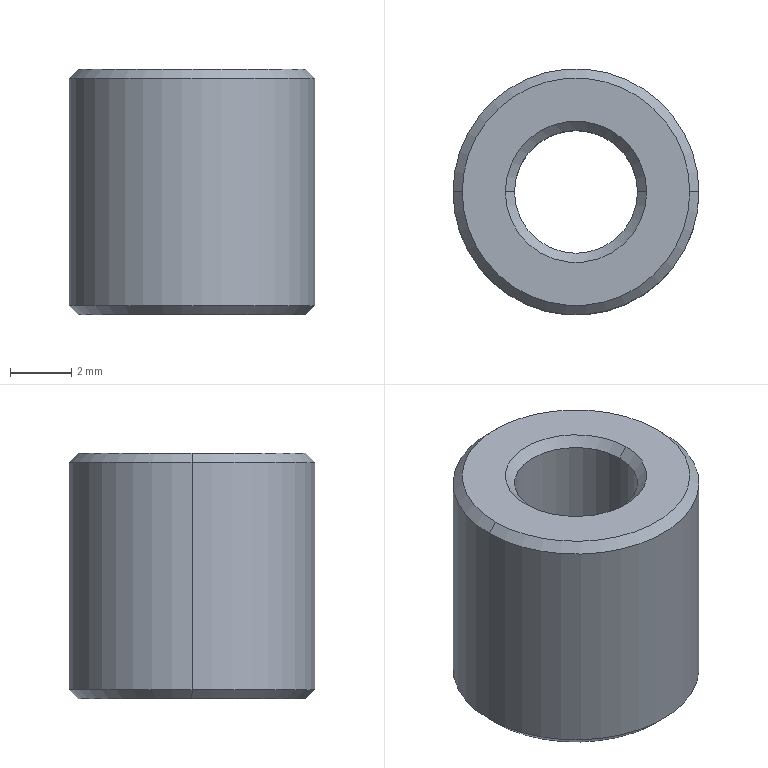Part | SolidWorks | features Chamfer 1, Extrusion 1 | 1 solid | 14 faces | box 8 x 8 x 8 mm | volume 298.2 mm3 | cone 8 | cylinder 4 | plane 2 | commonest cylinder face diameters 4 x2 8 x2
STEP:
#1=CARTESIAN_POINT('',(3.7,0.,8.));
#2=VERTEX_POINT('',#1);
#3=CARTESIAN_POINT('',(-3.7,0.,8.));
#4=VERTEX_POINT('',#3);
#5=CARTESIAN_POINT('',(0.,0.,8.));
#6=DIRECTION('',(0.,0.,1.));
#7=DIRECTION('',(1.,0.,0.));
#8=AXIS2_PLACEMENT_3D('',#5,#6,#7);
#9=CIRCLE('',#8,3.7);
#10=EDGE_CURVE('',#2,#4,#9,.T.);
#11=ORIENTED_EDGE('',*,*,#10,.F.);
#12=CARTESIAN_POINT('',(4.,0.,7.7));
#13=VERTEX_POINT('',#12);
#14=CARTESIAN_POINT('',(3.7,0.,8.));
#15=DIRECTION('',(0.7071,0.,-0.7071));
#16=VECTOR('',#15,1000.);
#17=LINE('',#14,#16);
#18=EDGE_CURVE('',#2,#13,#17,.T.);
#19=ORIENTED_EDGE('',*,*,#18,.T.);
#20=CARTESIAN_POINT('',(-4.,0.,7.7));
#21=VERTEX_POINT('',#20);
#22=CARTESIAN_POINT('',(0.,0.,7.7));
#23=DIRECTION('',(0.,0.,-1.));
#24=DIRECTION('',(1.,0.,0.));
#25=AXIS2_PLACEMENT_3D('',#22,#23,#24);
#26=CIRCLE('',#25,4.);
#27=EDGE_CURVE('',#21,#13,#26,.T.);
#28=ORIENTED_EDGE('',*,*,#27,.F.);
#29=CARTESIAN_POINT('',(-3.7,0.,8.));
#30=DIRECTION('',(-0.7071,0.,-0.7071));
#31=VECTOR('',#30,1000.);
#32=LINE('',#29,#31);
#33=EDGE_CURVE('',#4,#21,#32,.T.);
#34=ORIENTED_EDGE('',*,*,#33,.F.);
#35=EDGE_LOOP('',(#11,#19,#28,#34));
#36=FACE_OUTER_BOUND('',#35,.T.);
#37=CARTESIAN_POINT('',(0.,0.,8.));
#38=DIRECTION('',(0.,0.,-1.));
#39=DIRECTION('',(-1.,0.,0.));
#40=AXIS2_PLACEMENT_3D('',#37,#38,#39);
#41=CONICAL_SURFACE('',#40,3.7,0.7854);
#42=ADVANCED_FACE('',(#36),#41,.T.);
#43=CARTESIAN_POINT('',(-3.7,0.,0.));
#44=VERTEX_POINT('',#43);
#45=CARTESIAN_POINT('',(3.7,0.,0.));
#46=VERTEX_POINT('',#45);
#47=CARTESIAN_POINT('',(0.,0.,0.));
#48=DIRECTION('',(0.,0.,-1.));
#49=DIRECTION('',(1.,0.,0.));
#50=AXIS2_PLACEMENT_3D('',#47,#48,#49);
#51=CIRCLE('',#50,3.7);
#52=EDGE_CURVE('',#44,#46,#51,.T.);
#53=ORIENTED_EDGE('',*,*,#52,.F.);
#54=CARTESIAN_POINT('',(-4.,0.,0.3));
#55=VERTEX_POINT('',#54);
#56=CARTESIAN_POINT('',(-4.,0.,0.3));
#57=DIRECTION('',(-0.7071,0.,0.7071));
#58=VECTOR('',#57,1000.);
#59=LINE('',#56,#58);
#60=EDGE_CURVE('',#44,#55,#59,.T.);
#61=ORIENTED_EDGE('',*,*,#60,.T.);
#62=CARTESIAN_POINT('',(4.,0.,0.3));
#63=VERTEX_POINT('',#62);
#64=CARTESIAN_POINT('',(0.,0.,0.3));
#65=DIRECTION('',(0.,0.,1.));
#66=DIRECTION('',(1.,0.,0.));
#67=AXIS2_PLACEMENT_3D('',#64,#65,#66);
#68=CIRCLE('',#67,4.);
#69=EDGE_CURVE('',#63,#55,#68,.T.);
#70=ORIENTED_EDGE('',*,*,#69,.F.);
#71=CARTESIAN_POINT('',(4.,0.,0.3));
#72=DIRECTION('',(0.7071,0.,0.7071));
#73=VECTOR('',#72,1000.);
#74=LINE('',#71,#73);
#75=EDGE_CURVE('',#46,#63,#74,.T.);
#76=ORIENTED_EDGE('',*,*,#75,.F.);
#77=EDGE_LOOP('',(#53,#61,#70,#76));
#78=FACE_OUTER_BOUND('',#77,.T.);
#79=CARTESIAN_POINT('',(0.,0.,0.3));
#80=DIRECTION('',(0.,0.,1.));
#81=DIRECTION('',(1.,0.,0.));
#82=AXIS2_PLACEMENT_3D('',#79,#80,#81);
#83=CONICAL_SURFACE('',#82,4.,0.7854);
#84=ADVANCED_FACE('',(#78),#83,.T.);
#85=CARTESIAN_POINT('',(-2.,0.,7.7));
#86=VERTEX_POINT('',#85);
#87=CARTESIAN_POINT('',(2.,0.,7.7));
#88=VERTEX_POINT('',#87);
#89=CARTESIAN_POINT('',(0.,0.,7.7));
#90=DIRECTION('',(0.,0.,1.));
#91=DIRECTION('',(1.,0.,0.));
#92=AXIS2_PLACEMENT_3D('',#89,#90,#91);
#93=CIRCLE('',#92,2.);
#94=EDGE_CURVE('',#86,#88,#93,.T.);
#95=ORIENTED_EDGE('',*,*,#94,.F.);
#96=CARTESIAN_POINT('',(-2.3,0.,8.));
#97=VERTEX_POINT('',#96);
#98=CARTESIAN_POINT('',(-2.,0.,7.7));
#99=DIRECTION('',(-0.7071,0.,0.7071));
#100=VECTOR('',#99,1000.);
#101=LINE('',#98,#100);
#102=EDGE_CURVE('',#86,#97,#101,.T.);
#103=ORIENTED_EDGE('',*,*,#102,.T.);
#104=CARTESIAN_POINT('',(2.3,0.,8.));
#105=VERTEX_POINT('',#104);
#106=CARTESIAN_POINT('',(0.,0.,8.));
#107=DIRECTION('',(0.,0.,-1.));
#108=DIRECTION('',(1.,0.,0.));
#109=AXIS2_PLACEMENT_3D('',#106,#107,#108);
#110=CIRCLE('',#109,2.3);
#111=EDGE_CURVE('',#105,#97,#110,.T.);
#112=ORIENTED_EDGE('',*,*,#111,.F.);
#113=CARTESIAN_POINT('',(2.,0.,7.7));
#114=DIRECTION('',(0.7071,0.,0.7071));
#115=VECTOR('',#114,1000.);
#116=LINE('',#113,#115);
#117=EDGE_CURVE('',#88,#105,#116,.T.);
#118=ORIENTED_EDGE('',*,*,#117,.F.);
#119=EDGE_LOOP('',(#95,#103,#112,#118));
#120=FACE_OUTER_BOUND('',#119,.T.);
#121=CARTESIAN_POINT('',(0.,0.,7.7));
#122=DIRECTION('',(0.,0.,1.));
#123=DIRECTION('',(1.,0.,0.));
#124=AXIS2_PLACEMENT_3D('',#121,#122,#123);
#125=CONICAL_SURFACE('',#124,2.,0.7854);
#126=ADVANCED_FACE('',(#120),#125,.F.);
#127=CARTESIAN_POINT('',(2.,0.,0.3));
#128=VERTEX_POINT('',#127);
#129=CARTESIAN_POINT('',(-2.,0.,0.3));
#130=VERTEX_POINT('',#129);
#131=CARTESIAN_POINT('',(0.,0.,0.3));
#132=DIRECTION('',(0.,0.,-1.));
#133=DIRECTION('',(1.,0.,0.));
#134=AXIS2_PLACEMENT_3D('',#131,#132,#133);
#135=CIRCLE('',#134,2.);
#136=EDGE_CURVE('',#128,#130,#135,.T.);
#137=ORIENTED_EDGE('',*,*,#136,.F.);
#138=CARTESIAN_POINT('',(2.3,0.,0.));
#139=VERTEX_POINT('',#138);
#140=CARTESIAN_POINT('',(2.3,0.,0.));
#141=DIRECTION('',(0.7071,0.,-0.7071));
#142=VECTOR('',#141,1000.);
#143=LINE('',#140,#142);
#144=EDGE_CURVE('',#128,#139,#143,.T.);
#145=ORIENTED_EDGE('',*,*,#144,.T.);
#146=CARTESIAN_POINT('',(-2.3,0.,0.));
#147=VERTEX_POINT('',#146);
#148=CARTESIAN_POINT('',(0.,0.,0.));
#149=DIRECTION('',(0.,0.,1.));
#150=DIRECTION('',(1.,0.,0.));
#151=AXIS2_PLACEMENT_3D('',#148,#149,#150);
#152=CIRCLE('',#151,2.3);
#153=EDGE_CURVE('',#147,#139,#152,.T.);
#154=ORIENTED_EDGE('',*,*,#153,.F.);
#155=CARTESIAN_POINT('',(-2.3,0.,0.));
#156=DIRECTION('',(-0.7071,0.,-0.7071));
#157=VECTOR('',#156,1000.);
#158=LINE('',#155,#157);
#159=EDGE_CURVE('',#130,#147,#158,.T.);
#160=ORIENTED_EDGE('',*,*,#159,.F.);
#161=EDGE_LOOP('',(#137,#145,#154,#160));
#162=FACE_OUTER_BOUND('',#161,.T.);
#163=CARTESIAN_POINT('',(0.,0.,0.));
#164=DIRECTION('',(0.,0.,-1.));
#165=DIRECTION('',(-1.,0.,0.));
#166=AXIS2_PLACEMENT_3D('',#163,#164,#165);
#167=CONICAL_SURFACE('',#166,2.3,0.7854);
#168=ADVANCED_FACE('',(#162),#167,.F.);
#169=ORIENTED_EDGE('',*,*,#94,.T.);
#170=CARTESIAN_POINT('',(2.,0.,8.));
#171=DIRECTION('',(0.,0.,-1.));
#172=VECTOR('',#171,1000.);
#173=LINE('',#170,#172);
#174=EDGE_CURVE('',#88,#128,#173,.T.);
#175=ORIENTED_EDGE('',*,*,#174,.T.);
#176=ORIENTED_EDGE('',*,*,#136,.T.);
#177=CARTESIAN_POINT('',(-2.,0.,8.));
#178=DIRECTION('',(0.,0.,-1.));
#179=VECTOR('',#178,1000.);
#180=LINE('',#177,#179);
#181=EDGE_CURVE('',#86,#130,#180,.T.);
#182=ORIENTED_EDGE('',*,*,#181,.F.);
#183=EDGE_LOOP('',(#169,#175,#176,#182));
#184=FACE_OUTER_BOUND('',#183,.T.);
#185=CARTESIAN_POINT('',(0.,0.,8.));
#186=DIRECTION('',(0.,0.,-1.));
#187=DIRECTION('',(-1.,0.,0.));
#188=AXIS2_PLACEMENT_3D('',#185,#186,#187);
#189=CYLINDRICAL_SURFACE('',#188,2.);
#190=ADVANCED_FACE('',(#184),#189,.F.);
#191=ORIENTED_EDGE('',*,*,#27,.T.);
#192=CARTESIAN_POINT('',(4.,0.,8.));
#193=DIRECTION('',(0.,0.,-1.));
#194=VECTOR('',#193,1000.);
#195=LINE('',#192,#194);
#196=EDGE_CURVE('',#13,#63,#195,.T.);
#197=ORIENTED_EDGE('',*,*,#196,.T.);
#198=ORIENTED_EDGE('',*,*,#69,.T.);
#199=CARTESIAN_POINT('',(-4.,0.,8.));
#200=DIRECTION('',(0.,0.,-1.));
#201=VECTOR('',#200,1000.);
#202=LINE('',#199,#201);
#203=EDGE_CURVE('',#21,#55,#202,.T.);
#204=ORIENTED_EDGE('',*,*,#203,.F.);
#205=EDGE_LOOP('',(#191,#197,#198,#204));
#206=FACE_OUTER_BOUND('',#205,.T.);
#207=CARTESIAN_POINT('',(0.,0.,8.));
#208=DIRECTION('',(0.,0.,-1.));
#209=DIRECTION('',(-1.,0.,0.));
#210=AXIS2_PLACEMENT_3D('',#207,#208,#209);
#211=CYLINDRICAL_SURFACE('',#210,4.);
#212=ADVANCED_FACE('',(#206),#211,.T.);
#213=ORIENTED_EDGE('',*,*,#111,.T.);
#214=CARTESIAN_POINT('',(0.,0.,8.));
#215=DIRECTION('',(0.,0.,-1.));
#216=DIRECTION('',(1.,0.,0.));
#217=AXIS2_PLACEMENT_3D('',#214,#215,#216);
#218=CIRCLE('',#217,2.3);
#219=EDGE_CURVE('',#97,#105,#218,.T.);
#220=ORIENTED_EDGE('',*,*,#219,.T.);
#221=EDGE_LOOP('',(#213,#220));
#222=FACE_BOUND('',#221,.T.);
#223=CARTESIAN_POINT('',(0.,0.,8.));
#224=DIRECTION('',(0.,0.,1.));
#225=DIRECTION('',(1.,0.,0.));
#226=AXIS2_PLACEMENT_3D('',#223,#224,#225);
#227=CIRCLE('',#226,3.7);
#228=EDGE_CURVE('',#4,#2,#227,.T.);
#229=ORIENTED_EDGE('',*,*,#228,.T.);
#230=ORIENTED_EDGE('',*,*,#10,.T.);
#231=EDGE_LOOP('',(#229,#230));
#232=FACE_OUTER_BOUND('',#231,.T.);
#233=CARTESIAN_POINT('',(0.,0.,8.));
#234=DIRECTION('',(0.,0.,1.));
#235=DIRECTION('',(1.,0.,0.));
#236=AXIS2_PLACEMENT_3D('',#233,#234,#235);
#237=PLANE('',#236);
#238=ADVANCED_FACE('',(#222,#232),#237,.T.);
#239=ORIENTED_EDGE('',*,*,#153,.T.);
#240=CARTESIAN_POINT('',(0.,0.,0.));
#241=DIRECTION('',(0.,0.,1.));
#242=DIRECTION('',(1.,0.,0.));
#243=AXIS2_PLACEMENT_3D('',#240,#241,#242);
#244=CIRCLE('',#243,2.3);
#245=EDGE_CURVE('',#139,#147,#244,.T.);
#246=ORIENTED_EDGE('',*,*,#245,.T.);
#247=EDGE_LOOP('',(#239,#246));
#248=FACE_BOUND('',#247,.T.);
#249=CARTESIAN_POINT('',(0.,0.,0.));
#250=DIRECTION('',(0.,0.,-1.));
#251=DIRECTION('',(1.,0.,0.));
#252=AXIS2_PLACEMENT_3D('',#249,#250,#251);
#253=CIRCLE('',#252,3.7);
#254=EDGE_CURVE('',#46,#44,#253,.T.);
#255=ORIENTED_EDGE('',*,*,#254,.T.);
#256=ORIENTED_EDGE('',*,*,#52,.T.);
#257=EDGE_LOOP('',(#255,#256));
#258=FACE_OUTER_BOUND('',#257,.T.);
#259=CARTESIAN_POINT('',(0.,0.,0.));
#260=DIRECTION('',(0.,0.,1.));
#261=DIRECTION('',(1.,0.,0.));
#262=AXIS2_PLACEMENT_3D('',#259,#260,#261);
#263=PLANE('',#262);
#264=ADVANCED_FACE('',(#248,#258),#263,.F.);
#265=ORIENTED_EDGE('',*,*,#196,.F.);
#266=CARTESIAN_POINT('',(0.,0.,7.7));
#267=DIRECTION('',(0.,0.,-1.));
#268=DIRECTION('',(1.,0.,0.));
#269=AXIS2_PLACEMENT_3D('',#266,#267,#268);
#270=CIRCLE('',#269,4.);
#271=EDGE_CURVE('',#13,#21,#270,.T.);
#272=ORIENTED_EDGE('',*,*,#271,.T.);
#273=ORIENTED_EDGE('',*,*,#203,.T.);
#274=CARTESIAN_POINT('',(0.,0.,0.3));
#275=DIRECTION('',(0.,0.,1.));
#276=DIRECTION('',(1.,0.,0.));
#277=AXIS2_PLACEMENT_3D('',#274,#275,#276);
#278=CIRCLE('',#277,4.);
#279=EDGE_CURVE('',#55,#63,#278,.T.);
#280=ORIENTED_EDGE('',*,*,#279,.T.);
#281=EDGE_LOOP('',(#265,#272,#273,#280));
#282=FACE_OUTER_BOUND('',#281,.T.);
#283=CARTESIAN_POINT('',(0.,0.,8.));
#284=DIRECTION('',(0.,0.,-1.));
#285=DIRECTION('',(-1.,0.,0.));
#286=AXIS2_PLACEMENT_3D('',#283,#284,#285);
#287=CYLINDRICAL_SURFACE('',#286,4.);
#288=ADVANCED_FACE('',(#282),#287,.T.);
#289=ORIENTED_EDGE('',*,*,#174,.F.);
#290=CARTESIAN_POINT('',(0.,0.,7.7));
#291=DIRECTION('',(0.,0.,1.));
#292=DIRECTION('',(1.,0.,0.));
#293=AXIS2_PLACEMENT_3D('',#290,#291,#292);
#294=CIRCLE('',#293,2.);
#295=EDGE_CURVE('',#88,#86,#294,.T.);
#296=ORIENTED_EDGE('',*,*,#295,.T.);
#297=ORIENTED_EDGE('',*,*,#181,.T.);
#298=CARTESIAN_POINT('',(0.,0.,0.3));
#299=DIRECTION('',(0.,0.,-1.));
#300=DIRECTION('',(1.,0.,0.));
#301=AXIS2_PLACEMENT_3D('',#298,#299,#300);
#302=CIRCLE('',#301,2.);
#303=EDGE_CURVE('',#130,#128,#302,.T.);
#304=ORIENTED_EDGE('',*,*,#303,.T.);
#305=EDGE_LOOP('',(#289,#296,#297,#304));
#306=FACE_OUTER_BOUND('',#305,.T.);
#307=CARTESIAN_POINT('',(0.,0.,8.));
#308=DIRECTION('',(0.,0.,-1.));
#309=DIRECTION('',(-1.,0.,0.));
#310=AXIS2_PLACEMENT_3D('',#307,#308,#309);
#311=CYLINDRICAL_SURFACE('',#310,2.);
#312=ADVANCED_FACE('',(#306),#311,.F.);
#313=ORIENTED_EDGE('',*,*,#144,.F.);
#314=ORIENTED_EDGE('',*,*,#303,.F.);
#315=ORIENTED_EDGE('',*,*,#159,.T.);
#316=ORIENTED_EDGE('',*,*,#245,.F.);
#317=EDGE_LOOP('',(#313,#314,#315,#316));
#318=FACE_OUTER_BOUND('',#317,.T.);
#319=CARTESIAN_POINT('',(0.,0.,0.));
#320=DIRECTION('',(0.,0.,-1.));
#321=DIRECTION('',(-1.,0.,0.));
#322=AXIS2_PLACEMENT_3D('',#319,#320,#321);
#323=CONICAL_SURFACE('',#322,2.3,0.7854);
#324=ADVANCED_FACE('',(#318),#323,.F.);
#325=ORIENTED_EDGE('',*,*,#102,.F.);
#326=ORIENTED_EDGE('',*,*,#295,.F.);
#327=ORIENTED_EDGE('',*,*,#117,.T.);
#328=ORIENTED_EDGE('',*,*,#219,.F.);
#329=EDGE_LOOP('',(#325,#326,#327,#328));
#330=FACE_OUTER_BOUND('',#329,.T.);
#331=CARTESIAN_POINT('',(0.,0.,7.7));
#332=DIRECTION('',(0.,0.,1.));
#333=DIRECTION('',(1.,0.,0.));
#334=AXIS2_PLACEMENT_3D('',#331,#332,#333);
#335=CONICAL_SURFACE('',#334,2.,0.7854);
#336=ADVANCED_FACE('',(#330),#335,.F.);
#337=ORIENTED_EDGE('',*,*,#60,.F.);
#338=ORIENTED_EDGE('',*,*,#254,.F.);
#339=ORIENTED_EDGE('',*,*,#75,.T.);
#340=ORIENTED_EDGE('',*,*,#279,.F.);
#341=EDGE_LOOP('',(#337,#338,#339,#340));
#342=FACE_OUTER_BOUND('',#341,.T.);
#343=CARTESIAN_POINT('',(0.,0.,0.3));
#344=DIRECTION('',(0.,0.,1.));
#345=DIRECTION('',(1.,0.,0.));
#346=AXIS2_PLACEMENT_3D('',#343,#344,#345);
#347=CONICAL_SURFACE('',#346,4.,0.7854);
#348=ADVANCED_FACE('',(#342),#347,.T.);
#349=ORIENTED_EDGE('',*,*,#18,.F.);
#350=ORIENTED_EDGE('',*,*,#228,.F.);
#351=ORIENTED_EDGE('',*,*,#33,.T.);
#352=ORIENTED_EDGE('',*,*,#271,.F.);
#353=EDGE_LOOP('',(#349,#350,#351,#352));
#354=FACE_OUTER_BOUND('',#353,.T.);
#355=CARTESIAN_POINT('',(0.,0.,8.));
#356=DIRECTION('',(0.,0.,-1.));
#357=DIRECTION('',(-1.,0.,0.));
#358=AXIS2_PLACEMENT_3D('',#355,#356,#357);
#359=CONICAL_SURFACE('',#358,3.7,0.7854);
#360=ADVANCED_FACE('',(#354),#359,.T.);
#361=CLOSED_SHELL('',(#42,#84,#126,#168,#190,#212,#238,#264,#288,#312,#324,#336,#348,#360));
#362=MANIFOLD_SOLID_BREP('',#361);
#363=CARTESIAN_POINT('',(0.,0.,0.));
#364=DIRECTION('',(0.,0.,1.));
#365=DIRECTION('',(1.,0.,0.));
#366=AXIS2_PLACEMENT_3D('',#363,#364,#365);
#367=(LENGTH_UNIT()NAMED_UNIT(*)SI_UNIT(.MILLI.,.METRE.));
#368=UNCERTAINTY_MEASURE_WITH_UNIT(LENGTH_MEASURE(0.00001),#367,'','');
#369=(NAMED_UNIT(*)PLANE_ANGLE_UNIT()SI_UNIT($,.RADIAN.));
#370=(NAMED_UNIT(*)SI_UNIT($,.STERADIAN.)SOLID_ANGLE_UNIT());
#371=(GEOMETRIC_REPRESENTATION_CONTEXT(3)GLOBAL_UNCERTAINTY_ASSIGNED_CONTEXT((#368))GLOBAL_UNIT_ASSIGNED_CONTEXT((#367,#369,#370))REPRESENTATION_CONTEXT('',''));
#372=ADVANCED_BREP_SHAPE_REPRESENTATION('',(#362,#366),#371);